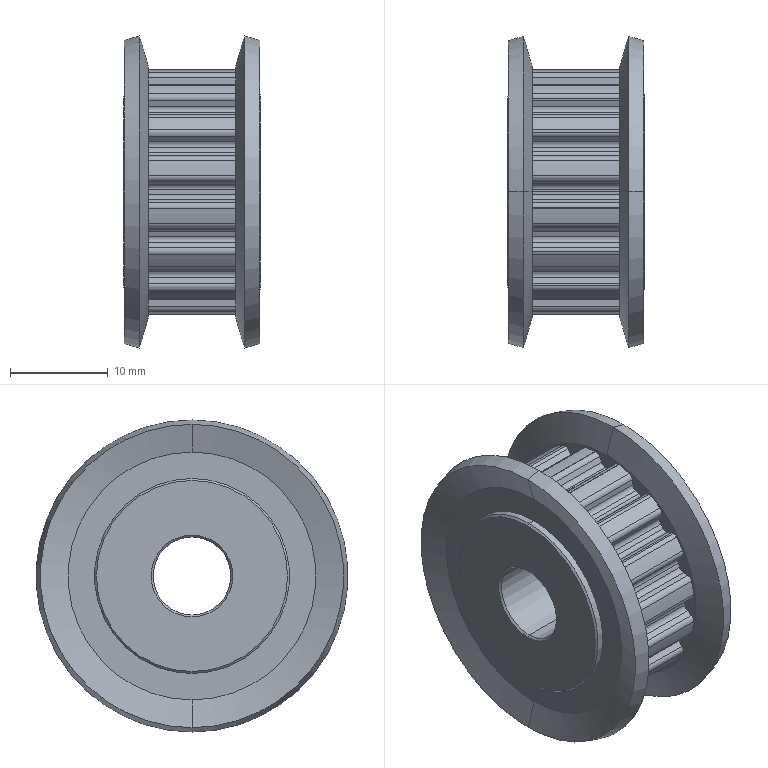Part | NX | features BREP 1 | 1 solid | 169 faces | box 14 x 32 x 32 mm | volume 6557 mm3 | cylinder 115 | plane 38 | cone 16 | commonest cylinder face diameters 1.22 x76 22.56 x17 25.36 x16 20 x4 8 x2